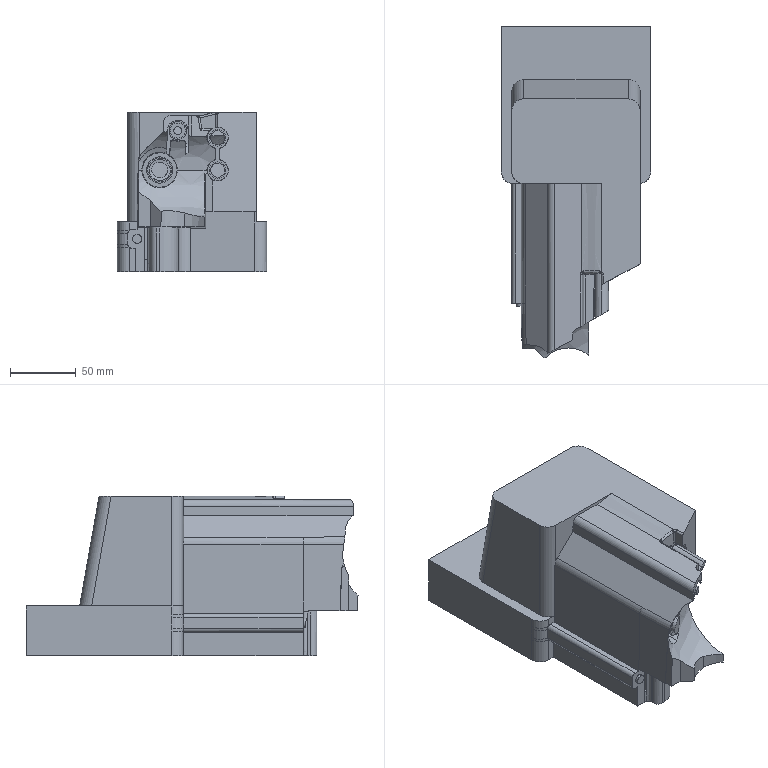Part | Creo | 1 solid | 169 faces | box 113.82 x 252.897 x 121.6 mm | volume 1876294 mm3 | plane 70 | cylinder 55 | cone 30 | spline 11 | torus 1 | sphere 1 | other 1 | commonest cylinder face diameters 18 x7 3.015 x6 10.653 x4 12.06 x4 12.663 x4 6.03 x3